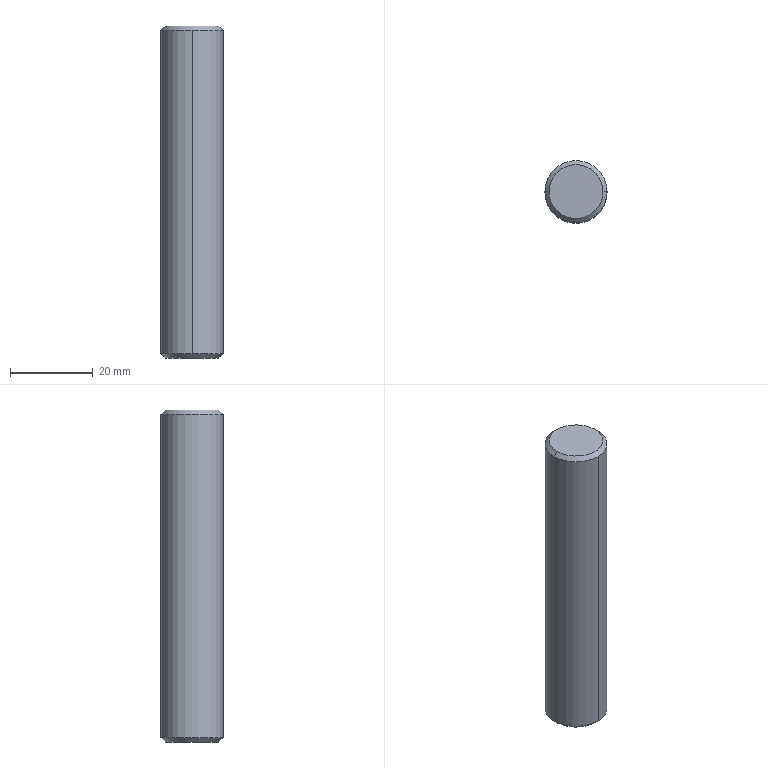Part | STEP file | 1 solid | 8 faces | box 15 x 15 x 80 mm | volume 14092 mm3 | cone 4 | cylinder 2 | plane 2 | commonest cylinder face diameters 15 x2
STEP:
#1=CARTESIAN_POINT('',(0.,0.,0.));
#2=DIRECTION('',(0.,0.,1.));
#3=DIRECTION('',(1.,0.,0.));
#4=AXIS2_PLACEMENT_3D('',#1,#2,#3);
#5=CARTESIAN_POINT('',(7.5,0.,-39.));
#6=VERTEX_POINT('',#5);
#7=CARTESIAN_POINT('',(0.,7.5,-39.));
#8=VERTEX_POINT('',#7);
#9=CARTESIAN_POINT('',(0.,0.,-39.));
#10=DIRECTION('',(0.,0.,1.));
#11=DIRECTION('',(0.,-1.,0.));
#12=AXIS2_PLACEMENT_3D('',#9,#10,#11);
#13=CIRCLE('',#12,7.5);
#14=CARTESIAN_POINT('',(0.,0.,40.));
#15=DIRECTION('',(0.,0.,1.));
#16=DIRECTION('',(0.,-1.,0.));
#17=AXIS2_PLACEMENT_3D('',#14,#15,#16);
#18=CYLINDRICAL_SURFACE('',#17,7.5);
#19=CARTESIAN_POINT('',(0.,-79.));
#20=DIRECTION('',(1.,0.));
#21=VECTOR('',#20,1.);
#22=LINE('',#19,#21);
#23=(GEOMETRIC_REPRESENTATION_CONTEXT(2)PARAMETRIC_REPRESENTATION_CONTEXT()REPRESENTATION_CONTEXT('',''));
#24=DEFINITIONAL_REPRESENTATION('',(#22),#23);
#25=PCURVE('',#18,#24);
#26=CARTESIAN_POINT('',(0.,0.,-39.));
#27=DIRECTION('',(0.,0.,1.));
#28=DIRECTION('',(1.,0.,0.));
#29=AXIS2_PLACEMENT_3D('',#26,#27,#28);
#30=CONICAL_SURFACE('',#29,7.5,0.7854);
#31=CARTESIAN_POINT('',(-1.571,0.));
#32=DIRECTION('',(1.,0.));
#33=VECTOR('',#32,1.);
#34=LINE('',#31,#33);
#35=(GEOMETRIC_REPRESENTATION_CONTEXT(2)PARAMETRIC_REPRESENTATION_CONTEXT()REPRESENTATION_CONTEXT('',''));
#36=DEFINITIONAL_REPRESENTATION('',(#34),#35);
#37=PCURVE('',#30,#36);
#38=SURFACE_CURVE('',#13,(#25,#37),.PCURVE_S1.);
#39=EDGE_CURVE('',#6,#8,#38,.T.);
#40=ORIENTED_EDGE('',*,*,#39,.T.);
#41=CARTESIAN_POINT('',(0.,7.5,39.));
#42=VERTEX_POINT('',#41);
#43=CARTESIAN_POINT('',(0.,7.5,40.));
#44=DIRECTION('',(0.,0.,1.));
#45=VECTOR('',#44,1.);
#46=LINE('',#43,#45);
#47=CARTESIAN_POINT('',(3.142,0.));
#48=DIRECTION('',(0.,1.));
#49=VECTOR('',#48,1.);
#50=LINE('',#47,#49);
#51=(GEOMETRIC_REPRESENTATION_CONTEXT(2)PARAMETRIC_REPRESENTATION_CONTEXT()REPRESENTATION_CONTEXT('',''));
#52=DEFINITIONAL_REPRESENTATION('',(#50),#51);
#53=PCURVE('',#18,#52);
#54=CARTESIAN_POINT('',(0.,0.,40.));
#55=DIRECTION('',(0.,0.,1.));
#56=DIRECTION('',(0.,-1.,0.));
#57=AXIS2_PLACEMENT_3D('',#54,#55,#56);
#58=CYLINDRICAL_SURFACE('',#57,7.5);
#59=CARTESIAN_POINT('',(3.142,0.));
#60=DIRECTION('',(0.,1.));
#61=VECTOR('',#60,1.);
#62=LINE('',#59,#61);
#63=(GEOMETRIC_REPRESENTATION_CONTEXT(2)PARAMETRIC_REPRESENTATION_CONTEXT()REPRESENTATION_CONTEXT('',''));
#64=DEFINITIONAL_REPRESENTATION('',(#62),#63);
#65=PCURVE('',#58,#64);
#66=SURFACE_CURVE('',#46,(#53,#65),.PCURVE_S1.);
#67=EDGE_CURVE('',#8,#42,#66,.T.);
#68=ORIENTED_EDGE('',*,*,#67,.T.);
#69=CARTESIAN_POINT('',(7.5,0.,39.));
#70=VERTEX_POINT('',#69);
#71=CARTESIAN_POINT('',(0.,0.,39.));
#72=DIRECTION('',(0.,0.,-1.));
#73=DIRECTION('',(0.,-1.,0.));
#74=AXIS2_PLACEMENT_3D('',#71,#72,#73);
#75=CIRCLE('',#74,7.5);
#76=CARTESIAN_POINT('',(6.283,-1.));
#77=DIRECTION('',(-1.,0.));
#78=VECTOR('',#77,1.);
#79=LINE('',#76,#78);
#80=(GEOMETRIC_REPRESENTATION_CONTEXT(2)PARAMETRIC_REPRESENTATION_CONTEXT()REPRESENTATION_CONTEXT('',''));
#81=DEFINITIONAL_REPRESENTATION('',(#79),#80);
#82=PCURVE('',#18,#81);
#83=CARTESIAN_POINT('',(0.,0.,39.));
#84=DIRECTION('',(0.,0.,-1.));
#85=DIRECTION('',(-1.,0.,0.));
#86=AXIS2_PLACEMENT_3D('',#83,#84,#85);
#87=CONICAL_SURFACE('',#86,7.5,0.7854);
#88=CARTESIAN_POINT('',(-1.571,0.));
#89=DIRECTION('',(1.,0.));
#90=VECTOR('',#89,1.);
#91=LINE('',#88,#90);
#92=(GEOMETRIC_REPRESENTATION_CONTEXT(2)PARAMETRIC_REPRESENTATION_CONTEXT()REPRESENTATION_CONTEXT('',''));
#93=DEFINITIONAL_REPRESENTATION('',(#91),#92);
#94=PCURVE('',#87,#93);
#95=SURFACE_CURVE('',#75,(#82,#94),.PCURVE_S1.);
#96=EDGE_CURVE('',#42,#70,#95,.T.);
#97=ORIENTED_EDGE('',*,*,#96,.T.);
#98=CARTESIAN_POINT('',(0.,-7.5,39.));
#99=VERTEX_POINT('',#98);
#100=CARTESIAN_POINT('',(0.,0.,39.));
#101=DIRECTION('',(0.,0.,-1.));
#102=DIRECTION('',(0.,-1.,0.));
#103=AXIS2_PLACEMENT_3D('',#100,#101,#102);
#104=CIRCLE('',#103,7.5);
#105=CARTESIAN_POINT('',(6.283,-1.));
#106=DIRECTION('',(-1.,0.));
#107=VECTOR('',#106,1.);
#108=LINE('',#105,#107);
#109=(GEOMETRIC_REPRESENTATION_CONTEXT(2)PARAMETRIC_REPRESENTATION_CONTEXT()REPRESENTATION_CONTEXT('',''));
#110=DEFINITIONAL_REPRESENTATION('',(#108),#109);
#111=PCURVE('',#18,#110);
#112=CARTESIAN_POINT('',(0.,0.,39.));
#113=DIRECTION('',(0.,0.,-1.));
#114=DIRECTION('',(-1.,0.,0.));
#115=AXIS2_PLACEMENT_3D('',#112,#113,#114);
#116=CONICAL_SURFACE('',#115,7.5,0.7854);
#117=CARTESIAN_POINT('',(-1.571,0.));
#118=DIRECTION('',(1.,0.));
#119=VECTOR('',#118,1.);
#120=LINE('',#117,#119);
#121=(GEOMETRIC_REPRESENTATION_CONTEXT(2)PARAMETRIC_REPRESENTATION_CONTEXT()REPRESENTATION_CONTEXT('',''));
#122=DEFINITIONAL_REPRESENTATION('',(#120),#121);
#123=PCURVE('',#116,#122);
#124=SURFACE_CURVE('',#104,(#111,#123),.PCURVE_S1.);
#125=EDGE_CURVE('',#70,#99,#124,.T.);
#126=ORIENTED_EDGE('',*,*,#125,.T.);
#127=CARTESIAN_POINT('',(0.,-7.5,-39.));
#128=VERTEX_POINT('',#127);
#129=CARTESIAN_POINT('',(0.,-7.5,40.));
#130=DIRECTION('',(0.,0.,1.));
#131=VECTOR('',#130,1.);
#132=LINE('',#129,#131);
#133=CARTESIAN_POINT('',(0.,0.));
#134=DIRECTION('',(0.,1.));
#135=VECTOR('',#134,1.);
#136=LINE('',#133,#135);
#137=(GEOMETRIC_REPRESENTATION_CONTEXT(2)PARAMETRIC_REPRESENTATION_CONTEXT()REPRESENTATION_CONTEXT('',''));
#138=DEFINITIONAL_REPRESENTATION('',(#136),#137);
#139=PCURVE('',#18,#138);
#140=CARTESIAN_POINT('',(6.283,0.));
#141=DIRECTION('',(0.,1.));
#142=VECTOR('',#141,1.);
#143=LINE('',#140,#142);
#144=(GEOMETRIC_REPRESENTATION_CONTEXT(2)PARAMETRIC_REPRESENTATION_CONTEXT()REPRESENTATION_CONTEXT('',''));
#145=DEFINITIONAL_REPRESENTATION('',(#143),#144);
#146=PCURVE('',#58,#145);
#147=SURFACE_CURVE('',#132,(#139,#146),.PCURVE_S1.);
#148=EDGE_CURVE('',#128,#99,#147,.T.);
#149=ORIENTED_EDGE('',*,*,#148,.F.);
#150=CARTESIAN_POINT('',(0.,0.,-39.));
#151=DIRECTION('',(0.,0.,1.));
#152=DIRECTION('',(0.,-1.,0.));
#153=AXIS2_PLACEMENT_3D('',#150,#151,#152);
#154=CIRCLE('',#153,7.5);
#155=CARTESIAN_POINT('',(0.,-79.));
#156=DIRECTION('',(1.,0.));
#157=VECTOR('',#156,1.);
#158=LINE('',#155,#157);
#159=(GEOMETRIC_REPRESENTATION_CONTEXT(2)PARAMETRIC_REPRESENTATION_CONTEXT()REPRESENTATION_CONTEXT('',''));
#160=DEFINITIONAL_REPRESENTATION('',(#158),#159);
#161=PCURVE('',#18,#160);
#162=CARTESIAN_POINT('',(0.,0.,-39.));
#163=DIRECTION('',(0.,0.,1.));
#164=DIRECTION('',(1.,0.,0.));
#165=AXIS2_PLACEMENT_3D('',#162,#163,#164);
#166=CONICAL_SURFACE('',#165,7.5,0.7854);
#167=CARTESIAN_POINT('',(4.712,0.));
#168=DIRECTION('',(1.,0.));
#169=VECTOR('',#168,1.);
#170=LINE('',#167,#169);
#171=(GEOMETRIC_REPRESENTATION_CONTEXT(2)PARAMETRIC_REPRESENTATION_CONTEXT()REPRESENTATION_CONTEXT('',''));
#172=DEFINITIONAL_REPRESENTATION('',(#170),#171);
#173=PCURVE('',#166,#172);
#174=SURFACE_CURVE('',#154,(#161,#173),.PCURVE_S1.);
#175=EDGE_CURVE('',#128,#6,#174,.T.);
#176=ORIENTED_EDGE('',*,*,#175,.T.);
#177=EDGE_LOOP('',(#40,#68,#97,#126,#149,#176));
#178=FACE_BOUND('',#177,.T.);
#179=ADVANCED_FACE('',(#178),#18,.T.);
#180=CARTESIAN_POINT('',(6.5,0.,-40.));
#181=VERTEX_POINT('',#180);
#182=CARTESIAN_POINT('',(-6.5,0.,-40.));
#183=VERTEX_POINT('',#182);
#184=CARTESIAN_POINT('',(0.,0.,-40.));
#185=DIRECTION('',(0.,0.,1.));
#186=DIRECTION('',(1.,0.,0.));
#187=AXIS2_PLACEMENT_3D('',#184,#185,#186);
#188=CIRCLE('',#187,6.5);
#189=CARTESIAN_POINT('',(0.,-1.));
#190=DIRECTION('',(1.,0.));
#191=VECTOR('',#190,1.);
#192=LINE('',#189,#191);
#193=(GEOMETRIC_REPRESENTATION_CONTEXT(2)PARAMETRIC_REPRESENTATION_CONTEXT()REPRESENTATION_CONTEXT('',''));
#194=DEFINITIONAL_REPRESENTATION('',(#192),#193);
#195=PCURVE('',#30,#194);
#196=CARTESIAN_POINT('',(0.,0.,-40.));
#197=DIRECTION('',(0.,0.,1.));
#198=DIRECTION('',(1.,0.,0.));
#199=AXIS2_PLACEMENT_3D('',#196,#197,#198);
#200=PLANE('',#199);
#201=CARTESIAN_POINT('',(0.,0.));
#202=DIRECTION('',(1.,0.));
#203=AXIS2_PLACEMENT_2D('',#201,#202);
#204=CIRCLE('',#203,6.5);
#205=(GEOMETRIC_REPRESENTATION_CONTEXT(2)PARAMETRIC_REPRESENTATION_CONTEXT()REPRESENTATION_CONTEXT('',''));
#206=DEFINITIONAL_REPRESENTATION('',(#204),#205);
#207=PCURVE('',#200,#206);
#208=SURFACE_CURVE('',#188,(#195,#207),.PCURVE_S1.);
#209=EDGE_CURVE('',#181,#183,#208,.T.);
#210=ORIENTED_EDGE('',*,*,#209,.T.);
#211=CARTESIAN_POINT('',(-7.5,0.,-39.));
#212=VERTEX_POINT('',#211);
#213=CARTESIAN_POINT('',(-7.5,0.,-39.));
#214=DIRECTION('',(-0.7071,0.,0.7071));
#215=VECTOR('',#214,1.);
#216=LINE('',#213,#215);
#217=CARTESIAN_POINT('',(3.142,0.));
#218=DIRECTION('',(0.,1.));
#219=VECTOR('',#218,1.);
#220=LINE('',#217,#219);
#221=(GEOMETRIC_REPRESENTATION_CONTEXT(2)PARAMETRIC_REPRESENTATION_CONTEXT()REPRESENTATION_CONTEXT('',''));
#222=DEFINITIONAL_REPRESENTATION('',(#220),#221);
#223=PCURVE('',#30,#222);
#224=CARTESIAN_POINT('',(3.142,0.));
#225=DIRECTION('',(0.,1.));
#226=VECTOR('',#225,1.);
#227=LINE('',#224,#226);
#228=(GEOMETRIC_REPRESENTATION_CONTEXT(2)PARAMETRIC_REPRESENTATION_CONTEXT()REPRESENTATION_CONTEXT('',''));
#229=DEFINITIONAL_REPRESENTATION('',(#227),#228);
#230=PCURVE('',#166,#229);
#231=SURFACE_CURVE('',#216,(#223,#230),.PCURVE_S1.);
#232=EDGE_CURVE('',#183,#212,#231,.T.);
#233=ORIENTED_EDGE('',*,*,#232,.T.);
#234=CARTESIAN_POINT('',(0.,0.,-39.));
#235=DIRECTION('',(0.,0.,1.));
#236=DIRECTION('',(0.,-1.,0.));
#237=AXIS2_PLACEMENT_3D('',#234,#235,#236);
#238=CIRCLE('',#237,7.5);
#239=CARTESIAN_POINT('',(-1.571,0.));
#240=DIRECTION('',(1.,0.));
#241=VECTOR('',#240,1.);
#242=LINE('',#239,#241);
#243=(GEOMETRIC_REPRESENTATION_CONTEXT(2)PARAMETRIC_REPRESENTATION_CONTEXT()REPRESENTATION_CONTEXT('',''));
#244=DEFINITIONAL_REPRESENTATION('',(#242),#243);
#245=PCURVE('',#30,#244);
#246=CARTESIAN_POINT('',(0.,-79.));
#247=DIRECTION('',(1.,0.));
#248=VECTOR('',#247,1.);
#249=LINE('',#246,#248);
#250=(GEOMETRIC_REPRESENTATION_CONTEXT(2)PARAMETRIC_REPRESENTATION_CONTEXT()REPRESENTATION_CONTEXT('',''));
#251=DEFINITIONAL_REPRESENTATION('',(#249),#250);
#252=PCURVE('',#58,#251);
#253=SURFACE_CURVE('',#238,(#245,#252),.PCURVE_S1.);
#254=EDGE_CURVE('',#8,#212,#253,.T.);
#255=ORIENTED_EDGE('',*,*,#254,.F.);
#256=ORIENTED_EDGE('',*,*,#39,.F.);
#257=CARTESIAN_POINT('',(7.5,0.,-39.));
#258=DIRECTION('',(0.7071,0.,0.7071));
#259=VECTOR('',#258,1.);
#260=LINE('',#257,#259);
#261=CARTESIAN_POINT('',(0.,0.));
#262=DIRECTION('',(0.,1.));
#263=VECTOR('',#262,1.);
#264=LINE('',#261,#263);
#265=(GEOMETRIC_REPRESENTATION_CONTEXT(2)PARAMETRIC_REPRESENTATION_CONTEXT()REPRESENTATION_CONTEXT('',''));
#266=DEFINITIONAL_REPRESENTATION('',(#264),#265);
#267=PCURVE('',#30,#266);
#268=CARTESIAN_POINT('',(6.283,0.));
#269=DIRECTION('',(0.,1.));
#270=VECTOR('',#269,1.);
#271=LINE('',#268,#270);
#272=(GEOMETRIC_REPRESENTATION_CONTEXT(2)PARAMETRIC_REPRESENTATION_CONTEXT()REPRESENTATION_CONTEXT('',''));
#273=DEFINITIONAL_REPRESENTATION('',(#271),#272);
#274=PCURVE('',#166,#273);
#275=SURFACE_CURVE('',#260,(#267,#274),.PCURVE_S1.);
#276=EDGE_CURVE('',#181,#6,#275,.T.);
#277=ORIENTED_EDGE('',*,*,#276,.F.);
#278=EDGE_LOOP('',(#210,#233,#255,#256,#277));
#279=FACE_BOUND('',#278,.T.);
#280=ADVANCED_FACE('',(#279),#30,.T.);
#281=CARTESIAN_POINT('',(-6.5,0.,40.));
#282=VERTEX_POINT('',#281);
#283=CARTESIAN_POINT('',(6.5,0.,40.));
#284=VERTEX_POINT('',#283);
#285=CARTESIAN_POINT('',(0.,0.,40.));
#286=DIRECTION('',(0.,0.,-1.));
#287=DIRECTION('',(-1.,0.,0.));
#288=AXIS2_PLACEMENT_3D('',#285,#286,#287);
#289=CIRCLE('',#288,6.5);
#290=CARTESIAN_POINT('',(0.,-1.));
#291=DIRECTION('',(1.,0.));
#292=VECTOR('',#291,1.);
#293=LINE('',#290,#292);
#294=(GEOMETRIC_REPRESENTATION_CONTEXT(2)PARAMETRIC_REPRESENTATION_CONTEXT()REPRESENTATION_CONTEXT('',''));
#295=DEFINITIONAL_REPRESENTATION('',(#293),#294);
#296=PCURVE('',#87,#295);
#297=CARTESIAN_POINT('',(0.,0.,40.));
#298=DIRECTION('',(0.,0.,1.));
#299=DIRECTION('',(1.,0.,0.));
#300=AXIS2_PLACEMENT_3D('',#297,#298,#299);
#301=PLANE('',#300);
#302=CARTESIAN_POINT('',(-6.5,0.));
#303=CARTESIAN_POINT('',(-6.5,11.258));
#304=CARTESIAN_POINT('',(3.25,5.629));
#305=CARTESIAN_POINT('',(13.,0.));
#306=CARTESIAN_POINT('',(3.25,-5.629));
#307=CARTESIAN_POINT('',(-6.5,-11.258));
#308=CARTESIAN_POINT('',(-6.5,0.));
#309=(BOUNDED_CURVE()B_SPLINE_CURVE(2,(#302,#303,#304,#305,#306,#307,#308),.UNSPECIFIED.,.T.,.F.)B_SPLINE_CURVE_WITH_KNOTS((1,2,2,2,2,1),(-2.094,0.,2.094,4.189,6.283,8.378),.UNSPECIFIED.)CURVE()GEOMETRIC_REPRESENTATION_ITEM()RATIONAL_B_SPLINE_CURVE((1.,0.5,1.,0.5,1.,0.5,1.))REPRESENTATION_ITEM(''));
#310=(GEOMETRIC_REPRESENTATION_CONTEXT(2)PARAMETRIC_REPRESENTATION_CONTEXT()REPRESENTATION_CONTEXT('',''));
#311=DEFINITIONAL_REPRESENTATION('',(#309),#310);
#312=PCURVE('',#301,#311);
#313=SURFACE_CURVE('',#289,(#296,#312),.PCURVE_S1.);
#314=EDGE_CURVE('',#282,#284,#313,.T.);
#315=ORIENTED_EDGE('',*,*,#314,.T.);
#316=CARTESIAN_POINT('',(7.5,0.,39.));
#317=DIRECTION('',(0.7071,0.,-0.7071));
#318=VECTOR('',#317,1.);
#319=LINE('',#316,#318);
#320=CARTESIAN_POINT('',(3.142,0.));
#321=DIRECTION('',(0.,1.));
#322=VECTOR('',#321,1.);
#323=LINE('',#320,#322);
#324=(GEOMETRIC_REPRESENTATION_CONTEXT(2)PARAMETRIC_REPRESENTATION_CONTEXT()REPRESENTATION_CONTEXT('',''));
#325=DEFINITIONAL_REPRESENTATION('',(#323),#324);
#326=PCURVE('',#87,#325);
#327=CARTESIAN_POINT('',(3.142,0.));
#328=DIRECTION('',(0.,1.));
#329=VECTOR('',#328,1.);
#330=LINE('',#327,#329);
#331=(GEOMETRIC_REPRESENTATION_CONTEXT(2)PARAMETRIC_REPRESENTATION_CONTEXT()REPRESENTATION_CONTEXT('',''));
#332=DEFINITIONAL_REPRESENTATION('',(#330),#331);
#333=PCURVE('',#116,#332);
#334=SURFACE_CURVE('',#319,(#326,#333),.PCURVE_S1.);
#335=EDGE_CURVE('',#284,#70,#334,.T.);
#336=ORIENTED_EDGE('',*,*,#335,.T.);
#337=ORIENTED_EDGE('',*,*,#96,.F.);
#338=CARTESIAN_POINT('',(-7.5,0.,39.));
#339=VERTEX_POINT('',#338);
#340=CARTESIAN_POINT('',(0.,0.,39.));
#341=DIRECTION('',(0.,0.,-1.));
#342=DIRECTION('',(0.,-1.,0.));
#343=AXIS2_PLACEMENT_3D('',#340,#341,#342);
#344=CIRCLE('',#343,7.5);
#345=CARTESIAN_POINT('',(-1.571,0.));
#346=DIRECTION('',(1.,0.));
#347=VECTOR('',#346,1.);
#348=LINE('',#345,#347);
#349=(GEOMETRIC_REPRESENTATION_CONTEXT(2)PARAMETRIC_REPRESENTATION_CONTEXT()REPRESENTATION_CONTEXT('',''));
#350=DEFINITIONAL_REPRESENTATION('',(#348),#349);
#351=PCURVE('',#87,#350);
#352=CARTESIAN_POINT('',(6.283,-1.));
#353=DIRECTION('',(-1.,0.));
#354=VECTOR('',#353,1.);
#355=LINE('',#352,#354);
#356=(GEOMETRIC_REPRESENTATION_CONTEXT(2)PARAMETRIC_REPRESENTATION_CONTEXT()REPRESENTATION_CONTEXT('',''));
#357=DEFINITIONAL_REPRESENTATION('',(#355),#356);
#358=PCURVE('',#58,#357);
#359=SURFACE_CURVE('',#344,(#351,#358),.PCURVE_S1.);
#360=EDGE_CURVE('',#339,#42,#359,.T.);
#361=ORIENTED_EDGE('',*,*,#360,.F.);
#362=CARTESIAN_POINT('',(-7.5,0.,39.));
#363=DIRECTION('',(-0.7071,0.,-0.7071));
#364=VECTOR('',#363,1.);
#365=LINE('',#362,#364);
#366=CARTESIAN_POINT('',(0.,0.));
#367=DIRECTION('',(0.,1.));
#368=VECTOR('',#367,1.);
#369=LINE('',#366,#368);
#370=(GEOMETRIC_REPRESENTATION_CONTEXT(2)PARAMETRIC_REPRESENTATION_CONTEXT()REPRESENTATION_CONTEXT('',''));
#371=DEFINITIONAL_REPRESENTATION('',(#369),#370);
#372=PCURVE('',#87,#371);
#373=CARTESIAN_POINT('',(6.283,0.));
#374=DIRECTION('',(0.,1.));
#375=VECTOR('',#374,1.);
#376=LINE('',#373,#375);
#377=(GEOMETRIC_REPRESENTATION_CONTEXT(2)PARAMETRIC_REPRESENTATION_CONTEXT()REPRESENTATION_CONTEXT('',''));
#378=DEFINITIONAL_REPRESENTATION('',(#376),#377);
#379=PCURVE('',#116,#378);
#380=SURFACE_CURVE('',#365,(#372,#379),.PCURVE_S1.);
#381=EDGE_CURVE('',#282,#339,#380,.T.);
#382=ORIENTED_EDGE('',*,*,#381,.F.);
#383=EDGE_LOOP('',(#315,#336,#337,#361,#382));
#384=FACE_BOUND('',#383,.T.);
#385=ADVANCED_FACE('',(#384),#87,.T.);
#386=ORIENTED_EDGE('',*,*,#67,.F.);
#387=ORIENTED_EDGE('',*,*,#254,.T.);
#388=CARTESIAN_POINT('',(0.,0.,-39.));
#389=DIRECTION('',(0.,0.,1.));
#390=DIRECTION('',(0.,-1.,0.));
#391=AXIS2_PLACEMENT_3D('',#388,#389,#390);
#392=CIRCLE('',#391,7.5);
#393=CARTESIAN_POINT('',(0.,-79.));
#394=DIRECTION('',(1.,0.));
#395=VECTOR('',#394,1.);
#396=LINE('',#393,#395);
#397=(GEOMETRIC_REPRESENTATION_CONTEXT(2)PARAMETRIC_REPRESENTATION_CONTEXT()REPRESENTATION_CONTEXT('',''));
#398=DEFINITIONAL_REPRESENTATION('',(#396),#397);
#399=PCURVE('',#58,#398);
#400=CARTESIAN_POINT('',(-1.571,0.));
#401=DIRECTION('',(1.,0.));
#402=VECTOR('',#401,1.);
#403=LINE('',#400,#402);
#404=(GEOMETRIC_REPRESENTATION_CONTEXT(2)PARAMETRIC_REPRESENTATION_CONTEXT()REPRESENTATION_CONTEXT('',''));
#405=DEFINITIONAL_REPRESENTATION('',(#403),#404);
#406=PCURVE('',#166,#405);
#407=SURFACE_CURVE('',#392,(#399,#406),.PCURVE_S1.);
#408=EDGE_CURVE('',#212,#128,#407,.T.);
#409=ORIENTED_EDGE('',*,*,#408,.T.);
#410=ORIENTED_EDGE('',*,*,#148,.T.);
#411=CARTESIAN_POINT('',(0.,0.,39.));
#412=DIRECTION('',(0.,0.,-1.));
#413=DIRECTION('',(0.,-1.,0.));
#414=AXIS2_PLACEMENT_3D('',#411,#412,#413);
#415=CIRCLE('',#414,7.5);
#416=CARTESIAN_POINT('',(6.283,-1.));
#417=DIRECTION('',(-1.,0.));
#418=VECTOR('',#417,1.);
#419=LINE('',#416,#418);
#420=(GEOMETRIC_REPRESENTATION_CONTEXT(2)PARAMETRIC_REPRESENTATION_CONTEXT()REPRESENTATION_CONTEXT('',''));
#421=DEFINITIONAL_REPRESENTATION('',(#419),#420);
#422=PCURVE('',#58,#421);
#423=CARTESIAN_POINT('',(4.712,0.));
#424=DIRECTION('',(1.,0.));
#425=VECTOR('',#424,1.);
#426=LINE('',#423,#425);
#427=(GEOMETRIC_REPRESENTATION_CONTEXT(2)PARAMETRIC_REPRESENTATION_CONTEXT()REPRESENTATION_CONTEXT('',''));
#428=DEFINITIONAL_REPRESENTATION('',(#426),#427);
#429=PCURVE('',#116,#428);
#430=SURFACE_CURVE('',#415,(#422,#429),.PCURVE_S1.);
#431=EDGE_CURVE('',#99,#339,#430,.T.);
#432=ORIENTED_EDGE('',*,*,#431,.T.);
#433=ORIENTED_EDGE('',*,*,#360,.T.);
#434=EDGE_LOOP('',(#386,#387,#409,#410,#432,#433));
#435=FACE_BOUND('',#434,.T.);
#436=ADVANCED_FACE('',(#435),#58,.T.);
#437=ORIENTED_EDGE('',*,*,#232,.F.);
#438=CARTESIAN_POINT('',(0.,0.,-40.));
#439=DIRECTION('',(0.,0.,1.));
#440=DIRECTION('',(1.,0.,0.));
#441=AXIS2_PLACEMENT_3D('',#438,#439,#440);
#442=CIRCLE('',#441,6.5);
#443=CARTESIAN_POINT('',(0.,-1.));
#444=DIRECTION('',(1.,0.));
#445=VECTOR('',#444,1.);
#446=LINE('',#443,#445);
#447=(GEOMETRIC_REPRESENTATION_CONTEXT(2)PARAMETRIC_REPRESENTATION_CONTEXT()REPRESENTATION_CONTEXT('',''));
#448=DEFINITIONAL_REPRESENTATION('',(#446),#447);
#449=PCURVE('',#166,#448);
#450=CARTESIAN_POINT('',(0.,0.));
#451=DIRECTION('',(1.,0.));
#452=AXIS2_PLACEMENT_2D('',#450,#451);
#453=CIRCLE('',#452,6.5);
#454=(GEOMETRIC_REPRESENTATION_CONTEXT(2)PARAMETRIC_REPRESENTATION_CONTEXT()REPRESENTATION_CONTEXT('',''));
#455=DEFINITIONAL_REPRESENTATION('',(#453),#454);
#456=PCURVE('',#200,#455);
#457=SURFACE_CURVE('',#442,(#449,#456),.PCURVE_S1.);
#458=EDGE_CURVE('',#183,#181,#457,.T.);
#459=ORIENTED_EDGE('',*,*,#458,.T.);
#460=ORIENTED_EDGE('',*,*,#276,.T.);
#461=ORIENTED_EDGE('',*,*,#175,.F.);
#462=ORIENTED_EDGE('',*,*,#408,.F.);
#463=EDGE_LOOP('',(#437,#459,#460,#461,#462));
#464=FACE_BOUND('',#463,.T.);
#465=ADVANCED_FACE('',(#464),#166,.T.);
#466=ORIENTED_EDGE('',*,*,#335,.F.);
#467=CARTESIAN_POINT('',(0.,0.,40.));
#468=DIRECTION('',(0.,0.,-1.));
#469=DIRECTION('',(-1.,0.,0.));
#470=AXIS2_PLACEMENT_3D('',#467,#468,#469);
#471=CIRCLE('',#470,6.5);
#472=CARTESIAN_POINT('',(0.,-1.));
#473=DIRECTION('',(1.,0.));
#474=VECTOR('',#473,1.);
#475=LINE('',#472,#474);
#476=(GEOMETRIC_REPRESENTATION_CONTEXT(2)PARAMETRIC_REPRESENTATION_CONTEXT()REPRESENTATION_CONTEXT('',''));
#477=DEFINITIONAL_REPRESENTATION('',(#475),#476);
#478=PCURVE('',#116,#477);
#479=CARTESIAN_POINT('',(-6.5,0.));
#480=CARTESIAN_POINT('',(-6.5,11.258));
#481=CARTESIAN_POINT('',(3.25,5.629));
#482=CARTESIAN_POINT('',(13.,0.));
#483=CARTESIAN_POINT('',(3.25,-5.629));
#484=CARTESIAN_POINT('',(-6.5,-11.258));
#485=CARTESIAN_POINT('',(-6.5,0.));
#486=(BOUNDED_CURVE()B_SPLINE_CURVE(2,(#479,#480,#481,#482,#483,#484,#485),.UNSPECIFIED.,.T.,.F.)B_SPLINE_CURVE_WITH_KNOTS((1,2,2,2,2,1),(-2.094,0.,2.094,4.189,6.283,8.378),.UNSPECIFIED.)CURVE()GEOMETRIC_REPRESENTATION_ITEM()RATIONAL_B_SPLINE_CURVE((1.,0.5,1.,0.5,1.,0.5,1.))REPRESENTATION_ITEM(''));
#487=(GEOMETRIC_REPRESENTATION_CONTEXT(2)PARAMETRIC_REPRESENTATION_CONTEXT()REPRESENTATION_CONTEXT('',''));
#488=DEFINITIONAL_REPRESENTATION('',(#486),#487);
#489=PCURVE('',#301,#488);
#490=SURFACE_CURVE('',#471,(#478,#489),.PCURVE_S1.);
#491=EDGE_CURVE('',#284,#282,#490,.T.);
#492=ORIENTED_EDGE('',*,*,#491,.T.);
#493=ORIENTED_EDGE('',*,*,#381,.T.);
#494=ORIENTED_EDGE('',*,*,#431,.F.);
#495=ORIENTED_EDGE('',*,*,#125,.F.);
#496=EDGE_LOOP('',(#466,#492,#493,#494,#495));
#497=FACE_BOUND('',#496,.T.);
#498=ADVANCED_FACE('',(#497),#116,.T.);
#499=ORIENTED_EDGE('',*,*,#209,.F.);
#500=ORIENTED_EDGE('',*,*,#458,.F.);
#501=EDGE_LOOP('',(#499,#500));
#502=FACE_BOUND('',#501,.T.);
#503=ADVANCED_FACE('',(#502),#200,.F.);
#504=ORIENTED_EDGE('',*,*,#314,.F.);
#505=ORIENTED_EDGE('',*,*,#491,.F.);
#506=EDGE_LOOP('',(#504,#505));
#507=FACE_BOUND('',#506,.T.);
#508=ADVANCED_FACE('',(#507),#301,.T.);
#509=CLOSED_SHELL('',(#179,#280,#385,#436,#465,#498,#503,#508));
#510=MANIFOLD_SOLID_BREP('',#509);
#511=(LENGTH_UNIT()NAMED_UNIT(*)SI_UNIT(.MILLI.,.METRE.));
#512=UNCERTAINTY_MEASURE_WITH_UNIT(LENGTH_MEASURE(0.0000001),#511,'','');
#513=(NAMED_UNIT(*)PLANE_ANGLE_UNIT()SI_UNIT($,.RADIAN.));
#514=(NAMED_UNIT(*)SI_UNIT($,.STERADIAN.)SOLID_ANGLE_UNIT());
#515=(GEOMETRIC_REPRESENTATION_CONTEXT(3)GLOBAL_UNCERTAINTY_ASSIGNED_CONTEXT((#512))GLOBAL_UNIT_ASSIGNED_CONTEXT((#511,#513,#514))REPRESENTATION_CONTEXT('',''));
#516=ADVANCED_BREP_SHAPE_REPRESENTATION('',(#4,#510),#515);